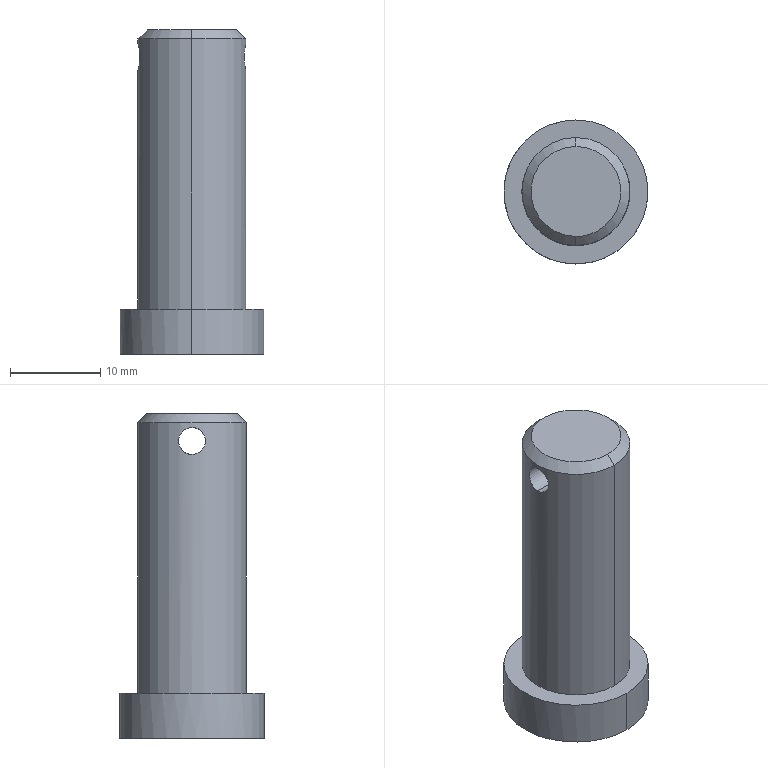Part | STEP file | Positioning_id1966_x_t | 1 solid | 11 faces | box 16 x 16 x 36 mm | volume 4409 mm3 | cylinder 6 | plane 3 | cone 2 | commonest cylinder face diameters 3 x2 12 x2 16 x2